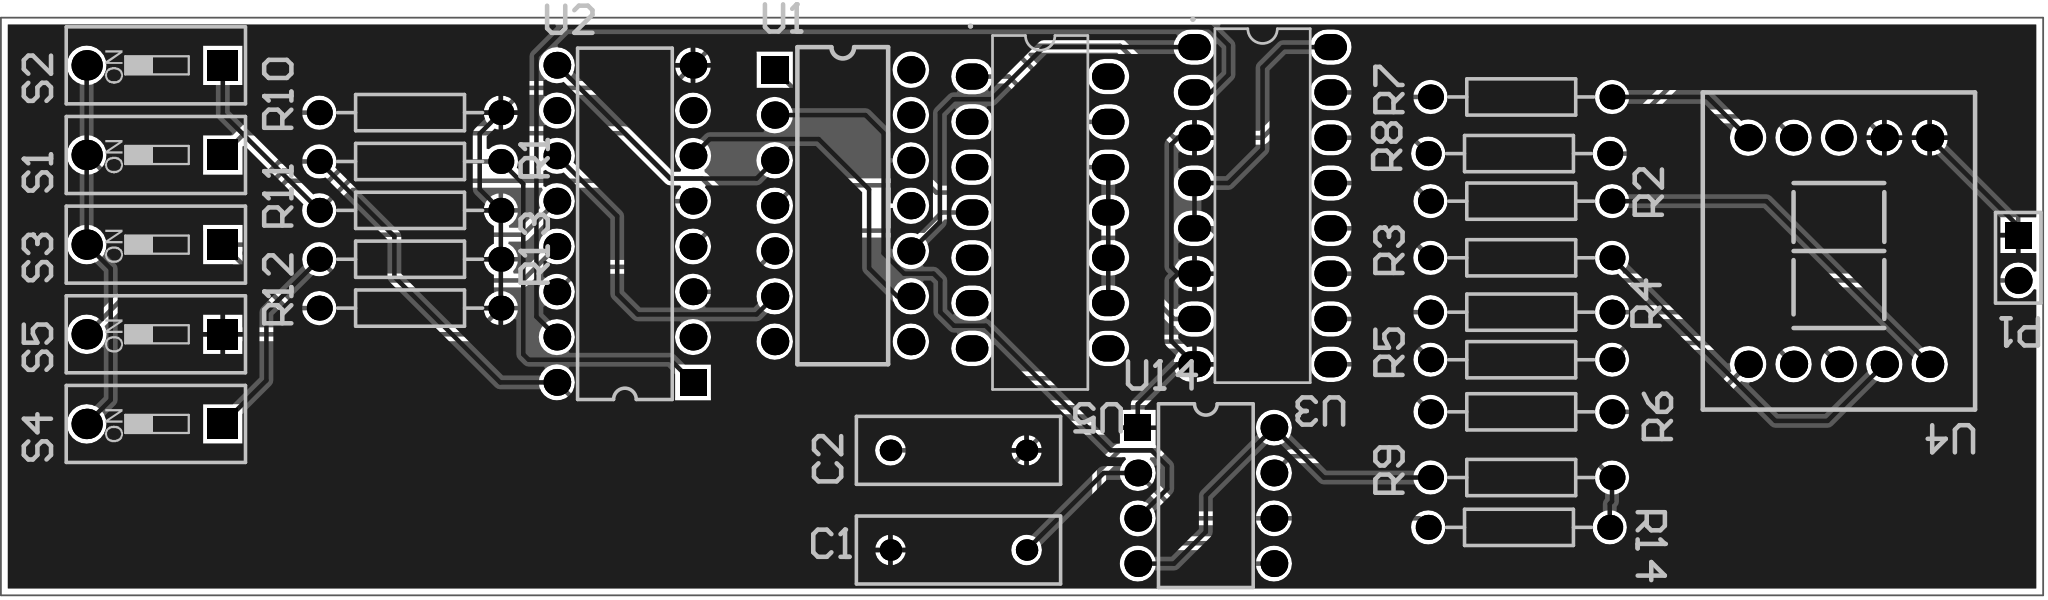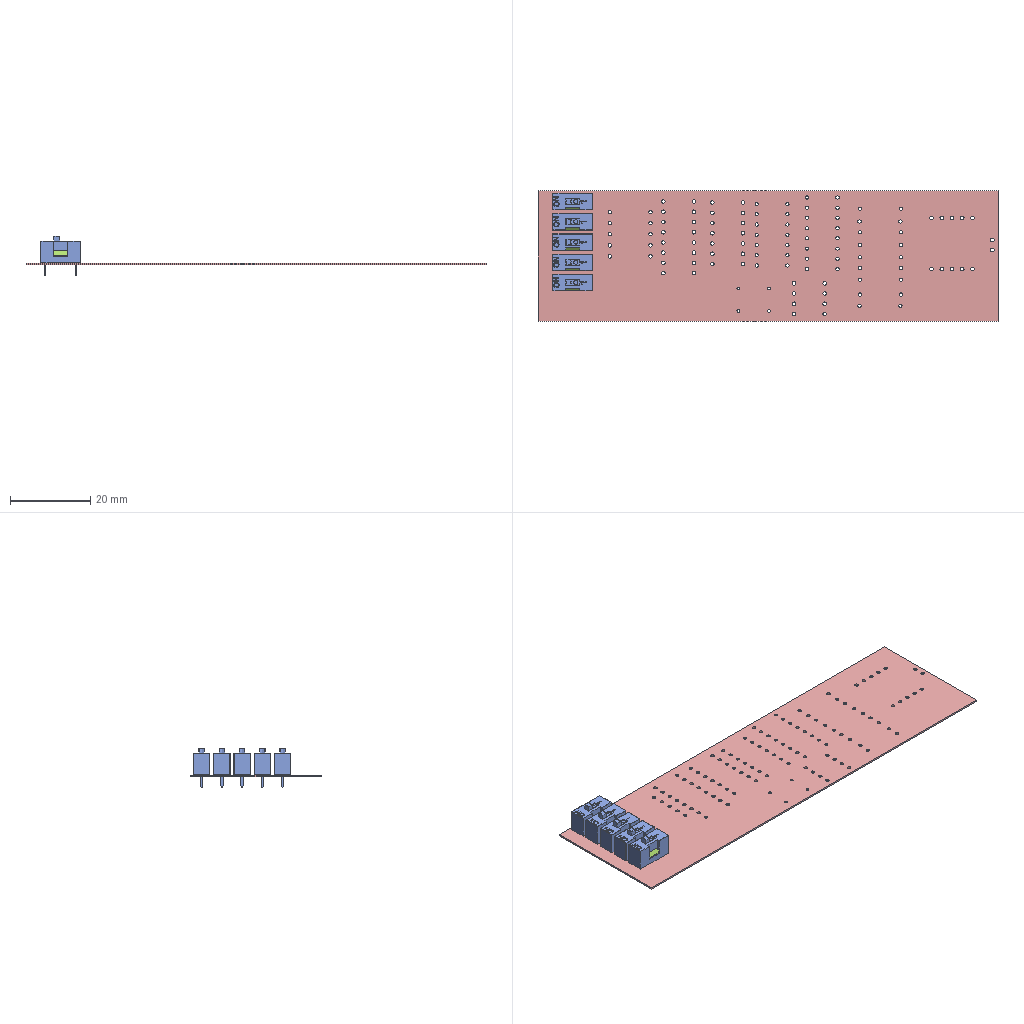Circuit board layout | Altium Designer | box 114.3 x 32.4 x 9.8 mm
Layer stack:
# Altium Designer layer stack of  (unit mm; dielectric type: 0 none, 1 core, 2 prepreg, 3 surface material)
index,name,kind,layer,copper_thickness_mm,dielectric_type,dielectric_thickness_mm,dielectric_material,dielectric_constant
0,Top Paste,other,,,,,,
1,Top Overlay,other,,,,,,
2,Top Solder,dielectric,,,3,0.0102,Solder Resist,3.5
3,Top Layer,copper,Top Layer,0.0356,,,,
4,Dielectric 1,dielectric,,,0,0.32,FR-4,4.8
5,Bottom Layer,copper,Bottom Layer,0.0356,,,,
6,Bottom Solder,dielectric,,,3,0.0102,Solder Resist,3.5
7,Bottom Overlay,other,,,,,,
8,Bottom Paste,other,,,,,,
# drill layer pairs: low layer,high layer
drill_pair,Top Layer,Bottom Layer
Part placement:
Designator,Comment,Layer,Footprint,Center-X(mm),Center-Y(mm),Rotation
U14,NE555,TopLayer,DIP-8-NE555,112.522,70.993,360
U5,CD4012,TopLayer,DIP14,103.251,86.868,270
U4,Single-digit LED display (common cathode),TopLayer,PCBComponent_1,147.955,84.709,180
U3,CD4511BCN,TopLayer,CD4511BCN,115.697,87.249,270
U2,SN74LS175N_1,TopLayer,N016,80.01,86.233,90
U1,CD4011,TopLayer,CD4011,92.202,87.249,360
S5,SW1-DIP2,TopLayer,DIP-1P,53.694,80.04,90
S4,SW1-DIP2,TopLayer,DIP-1P,53.694,75.014,90
S3,SW1-DIP2,TopLayer,DIP-1P,53.694,85.066,90
S2,SW1-DIP2,TopLayer,DIP-1P,53.694,95.118,90
S1,SW1-DIP2,TopLayer,DIP-1P,53.694,90.092,90
R14,Res2,TopLayer,AXIAL-0.4,130.048,69.215,360
R13,Res2,TopLayer,AXIAL-0.4,67.985,84.247,180
R12,Res2,TopLayer,AXIAL-0.4,67.985,81.507,180
R11,Res2,TopLayer,AXIAL-0.4,67.985,86.987,180
R10,Res2,TopLayer,AXIAL-0.4,67.985,92.467,180
R9,Res2,TopLayer,AXIAL-0.4,130.175,72.009,180
R8,Res2,TopLayer,AXIAL-0.4,130.048,90.17,180
R7,Res2,TopLayer,AXIAL-0.4,130.175,93.345,180
R6,Res2,TopLayer,AXIAL-0.4,130.175,75.692,180
R5,Res2,TopLayer,AXIAL-0.4,130.175,78.613,180
R4,Res2,TopLayer,AXIAL-0.4,130.175,81.28,180
R3,Res2,TopLayer,AXIAL-0.4,130.175,84.328,180
R2,Res2,TopLayer,AXIAL-0.4,130.175,87.503,180
R1,Res2,TopLayer,AXIAL-0.4,67.985,89.727,180
P1,Header 2,TopLayer,HDR1X2,157.988,84.328,270
C2,Cap,TopLayer,RAD-0.3,98.679,73.533,180
C1,Cap,TopLayer,RAD-0.3,98.679,67.945,360
Pad and via stacks:
# Altium Designer via and pad stacks of  (unit mm). Each distinct definition once, with the count of objects using it.
# via: kind,start_layer,end_layer,hole_mm,diameter_mm,mode(0 simple;1 top-mid-bottom;2 full stack),diameter_per_layer,count,example_net
# pad: kind,layer,hole_mm,hole_type(0 round;1 square;2 slot),plating,top_size,top_shape(1 round;2 rect;3 octagon;9 rounded rect),mid_size,bottom_size,mode,footprint,size_per_layer,count,example
pad,Multi-Layer,0.9,0,plated,1.5x1.5,2,1.5x1.5,1.5x1.5,0,HDR1X2,,1,P1.1
pad,Multi-Layer,0.9,0,plated,1.5x1.5,1,1.5x1.5,1.5x1.5,0,HDR1X2,,1,P1.2
pad,Multi-Layer,0.889,2,plated,1.524x1.524,1,1.524x1.524,1.524x1.524,0,CD4011,,13,U1.14
pad,Multi-Layer,0.889,2,plated,1.524x1.524,2,1.524x1.524,1.524x1.524,0,CD4011,,1,U1.1
pad,Multi-Layer,0.9,0,plated,1.7x1.7,2,1.7x1.7,1.7x1.7,0,DIP-1P,,5,S4.1
pad,Multi-Layer,0.9,0,plated,1.7x1.7,1,1.7x1.7,1.7x1.7,0,DIP-1P,,5,S4.2
pad,Multi-Layer,0.85,0,plated,1.4x1.4,1,1.4x1.4,1.4x1.4,0,AXIAL-0.4,,28,R1.1
pad,Multi-Layer,0.9,2,plated,1.5x1.5,2,1.5x1.5,1.5x1.5,0,N016,,1,U2.1
pad,Multi-Layer,0.9,2,plated,1.5x1.5,1,1.5x1.5,1.5x1.5,0,N016,,15,U2.2
pad,Multi-Layer,0.8,0,plated,1.462x1.827,1,1.462x1.827,1.462x1.827,0,CD4511BCN,,16,U3.1
pad,Multi-Layer,0.9144,0,plated,1.524x1.524,1,1.524x1.524,1.524x1.524,0,PCBComponent_1,,10,U4.1
pad,Multi-Layer,0.8,0,plated,1.462x1.827,1,1.462x1.827,1.462x1.827,0,DIP14,,14,U5.1
pad,Multi-Layer,0.9,2,plated,1.5x1.5,1,1.5x1.5,1.5x1.5,0,DIP-8-NE555,,7,U14.5
pad,Multi-Layer,0.9,2,plated,1.5x1.5,2,1.5x1.5,1.5x1.5,0,DIP-8-NE555,,1,U14.1
pad,Multi-Layer,0.7,0,plated,1.2x1.2,1,1.2x1.2,1.2x1.2,0,RAD-0.3,,4,C1.2
Copper pours:
name,layer,net,type(0 solid;1 hatched;2 none)
Top Layer-No Net,Top Layer,GND,0
Top Layer-No Net,Bottom Layer,GND,0
Design rules, without the lines most boards share:
# Altium Designer design rules of  (exported by Altium Designer, unit mm)
# columns: name | kind | enabled | priority | scope1 | scope2 | descriptor | typed fields (field=value)
Clearance | 0 | enabled | 1 | All | All | Clearance Constraint (Gap=10mil) (All),(All) | gap=0.254
PlaneConnect | 6 | enabled | 1 | All | All | Power Plane Connect Rule(Relief Connect )(Expansion=20mil) (Conductor Width=10mil) (Air Gap=10mil) (Entries=4) (All) | relief_conductor_width=0.254 relief_entries=4 relief_expansion=0.508
PolygonConnect | 20 | enabled | 1 | All | All | Polygon Connect Rule(Relief Connect )(Conductor Width=10mil) (Relief Angle=90 Angle) (Entries=4) (Air Gap Width=10mil) (All),(All) | connect_style(0=relief,1=direct,2=none)=0 relief_conductor_width=0.254 relief_entries=4
Width | 2 | enabled | 1 | All | All | Width Constraint (Min=10mil) (Max=10mil) (Preferred=10mil) (All) |
RoutingVias | 11 | enabled | 1 | All | All | Routing Via (MinHoleWidth=28mil) (MaxHoleWidth=28mil) (PreferredHoleWidth=28mil) (MinWidth=50mil) (MaxWidth=50mil) (PreferedWidth=50mil) (All) | via_min_hole=0.7112 via_max_hole=0.7112 via_preferred_diameter=1.27 via_preferred_hole=0.7112
PasteMaskExpansion | 14 | enabled | 1 | All | All | Paste Mask Expansion (Expansion =0mil) (All) | expansion=0
SolderMaskExpansion | 13 | enabled | 1 | All | All | Solder Mask Expansion (Expansion =4mil) (All) | expansion=0.1016
DiffPairsRouting | 51 | enabled | 1 | All | All | Differential Pairs Uncoupled Length using the Gap Constraints (Min=10mil) (Max=10mil) (Prefered=10mil)  and Width Constraints (Min=15mil) (Max=15mil) (Prefered=15mil) (All) |
HoleToHoleClearance | 52 | enabled | 1 | All | All | Hole To Hole Clearance (Gap=10mil) (All),(All) | gap=0.254
Classes set for this board:
# Altium Designer classes of  (member kind: 0 net, 1 component, 2 from-to, 3 pad, 4 layer, 5 differential pair, 6 design channel, 7 polygon, 8 structure, 9 xSignal)
# columns: class name | member kind | superclass | members
Sheet1 | 1 | no | C1; C2; P1; R1; R2; R3; R4; R5; R6; R7; R8; R9; R10; R11; R12; R13; R14; S1; S2; S3; S4; S5; U1; U2; U3; U4; U5; U14;